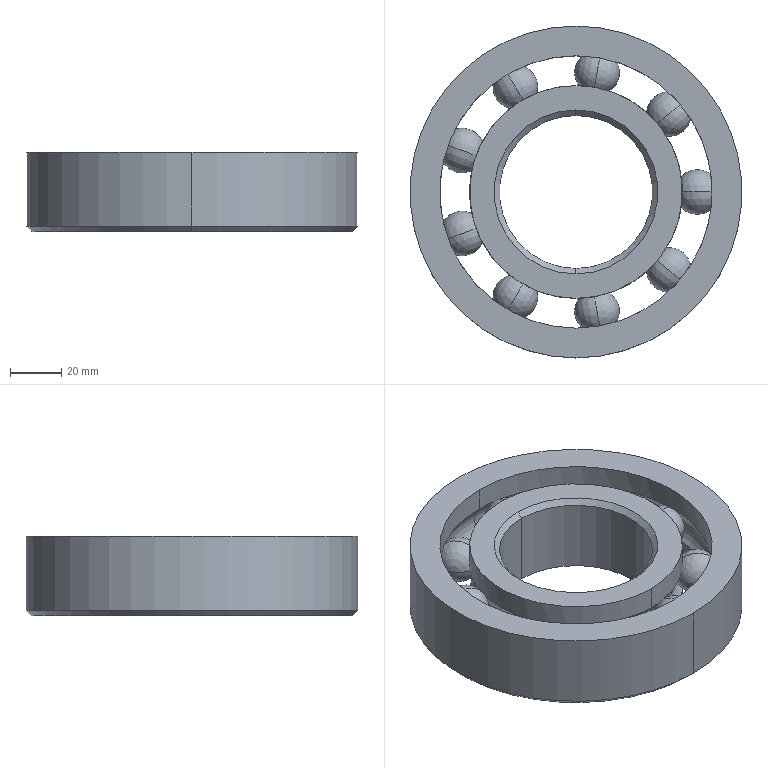Part | SolidWorks | features BaseBody 1 | 1 solid | 86 faces | box 130 x 130 x 31 mm | volume 224912 mm3 | sphere 36 | torus 30 | cylinder 12 | cone 4 | plane 4 | commonest cylinder face diameters 83.333 x4 106.667 x4 60 x2 130 x2